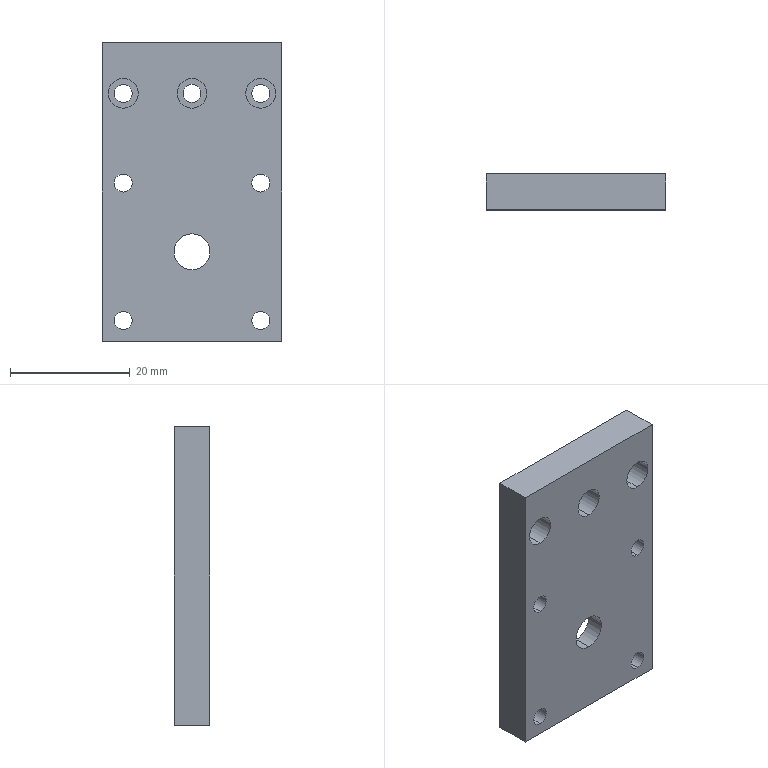Part | SolidWorks | features ICE 3, Cut 2, FlatPattern 1, SMBaseFlange 1, SheetMetal 1 | 1 solid | 34 faces | box 30 x 6 x 50 mm | volume 7901 mm3 | cylinder 24 | plane 10 | commonest cylinder face diameters 3 x14 5 x6 6 x2 15.5 x2
STEP:
#1=CARTESIAN_POINT('',(0.,-6.,14.));
#2=VERTEX_POINT('',#1);
#3=CARTESIAN_POINT('',(0.,-6.,19.));
#4=VERTEX_POINT('',#3);
#5=CARTESIAN_POINT('',(0.,-6.,16.5));
#6=DIRECTION('',(0.,1.,0.));
#7=DIRECTION('',(0.,0.,1.));
#8=AXIS2_PLACEMENT_3D('',#5,#6,#7);
#9=CIRCLE('',#8,2.5);
#10=EDGE_CURVE('',#2,#4,#9,.T.);
#11=ORIENTED_EDGE('',*,*,#10,.F.);
#12=CARTESIAN_POINT('',(0.,-2.,14.));
#13=VERTEX_POINT('',#12);
#14=CARTESIAN_POINT('',(0.,-6.,14.));
#15=DIRECTION('',(0.,1.,0.));
#16=VECTOR('',#15,1000.);
#17=LINE('',#14,#16);
#18=EDGE_CURVE('',#2,#13,#17,.T.);
#19=ORIENTED_EDGE('',*,*,#18,.T.);
#20=CARTESIAN_POINT('',(0.,-2.,19.));
#21=VERTEX_POINT('',#20);
#22=CARTESIAN_POINT('',(0.,-2.,16.5));
#23=DIRECTION('',(0.,1.,0.));
#24=DIRECTION('',(0.,0.,1.));
#25=AXIS2_PLACEMENT_3D('',#22,#23,#24);
#26=CIRCLE('',#25,2.5);
#27=EDGE_CURVE('',#13,#21,#26,.T.);
#28=ORIENTED_EDGE('',*,*,#27,.T.);
#29=CARTESIAN_POINT('',(0.,-6.,19.));
#30=DIRECTION('',(0.,1.,0.));
#31=VECTOR('',#30,1000.);
#32=LINE('',#29,#31);
#33=EDGE_CURVE('',#4,#21,#32,.T.);
#34=ORIENTED_EDGE('',*,*,#33,.F.);
#35=EDGE_LOOP('',(#11,#19,#28,#34));
#36=FACE_OUTER_BOUND('',#35,.T.);
#37=CARTESIAN_POINT('',(0.,-6.,16.5));
#38=DIRECTION('',(0.,1.,0.));
#39=DIRECTION('',(0.,0.,1.));
#40=AXIS2_PLACEMENT_3D('',#37,#38,#39);
#41=CYLINDRICAL_SURFACE('',#40,2.5);
#42=ADVANCED_FACE('',(#36),#41,.F.);
#43=CARTESIAN_POINT('',(11.5,-6.,14.));
#44=VERTEX_POINT('',#43);
#45=CARTESIAN_POINT('',(11.5,-6.,19.));
#46=VERTEX_POINT('',#45);
#47=CARTESIAN_POINT('',(11.5,-6.,16.5));
#48=DIRECTION('',(0.,1.,0.));
#49=DIRECTION('',(0.,0.,1.));
#50=AXIS2_PLACEMENT_3D('',#47,#48,#49);
#51=CIRCLE('',#50,2.5);
#52=EDGE_CURVE('',#44,#46,#51,.T.);
#53=ORIENTED_EDGE('',*,*,#52,.F.);
#54=CARTESIAN_POINT('',(11.5,-2.,14.));
#55=VERTEX_POINT('',#54);
#56=CARTESIAN_POINT('',(11.5,-6.,14.));
#57=DIRECTION('',(0.,1.,0.));
#58=VECTOR('',#57,1000.);
#59=LINE('',#56,#58);
#60=EDGE_CURVE('',#44,#55,#59,.T.);
#61=ORIENTED_EDGE('',*,*,#60,.T.);
#62=CARTESIAN_POINT('',(11.5,-2.,19.));
#63=VERTEX_POINT('',#62);
#64=CARTESIAN_POINT('',(11.5,-2.,16.5));
#65=DIRECTION('',(0.,1.,0.));
#66=DIRECTION('',(0.,0.,1.));
#67=AXIS2_PLACEMENT_3D('',#64,#65,#66);
#68=CIRCLE('',#67,2.5);
#69=EDGE_CURVE('',#55,#63,#68,.T.);
#70=ORIENTED_EDGE('',*,*,#69,.T.);
#71=CARTESIAN_POINT('',(11.5,-6.,19.));
#72=DIRECTION('',(0.,1.,0.));
#73=VECTOR('',#72,1000.);
#74=LINE('',#71,#73);
#75=EDGE_CURVE('',#46,#63,#74,.T.);
#76=ORIENTED_EDGE('',*,*,#75,.F.);
#77=EDGE_LOOP('',(#53,#61,#70,#76));
#78=FACE_OUTER_BOUND('',#77,.T.);
#79=CARTESIAN_POINT('',(11.5,-6.,16.5));
#80=DIRECTION('',(0.,1.,0.));
#81=DIRECTION('',(0.,0.,1.));
#82=AXIS2_PLACEMENT_3D('',#79,#80,#81);
#83=CYLINDRICAL_SURFACE('',#82,2.5);
#84=ADVANCED_FACE('',(#78),#83,.F.);
#85=CARTESIAN_POINT('',(-11.5,-6.,14.));
#86=VERTEX_POINT('',#85);
#87=CARTESIAN_POINT('',(-11.5,-6.,19.));
#88=VERTEX_POINT('',#87);
#89=CARTESIAN_POINT('',(-11.5,-6.,16.5));
#90=DIRECTION('',(0.,1.,0.));
#91=DIRECTION('',(0.,0.,1.));
#92=AXIS2_PLACEMENT_3D('',#89,#90,#91);
#93=CIRCLE('',#92,2.5);
#94=EDGE_CURVE('',#86,#88,#93,.T.);
#95=ORIENTED_EDGE('',*,*,#94,.F.);
#96=CARTESIAN_POINT('',(-11.5,-2.,14.));
#97=VERTEX_POINT('',#96);
#98=CARTESIAN_POINT('',(-11.5,-6.,14.));
#99=DIRECTION('',(0.,1.,0.));
#100=VECTOR('',#99,1000.);
#101=LINE('',#98,#100);
#102=EDGE_CURVE('',#86,#97,#101,.T.);
#103=ORIENTED_EDGE('',*,*,#102,.T.);
#104=CARTESIAN_POINT('',(-11.5,-2.,19.));
#105=VERTEX_POINT('',#104);
#106=CARTESIAN_POINT('',(-11.5,-2.,16.5));
#107=DIRECTION('',(0.,1.,0.));
#108=DIRECTION('',(0.,0.,1.));
#109=AXIS2_PLACEMENT_3D('',#106,#107,#108);
#110=CIRCLE('',#109,2.5);
#111=EDGE_CURVE('',#97,#105,#110,.T.);
#112=ORIENTED_EDGE('',*,*,#111,.T.);
#113=CARTESIAN_POINT('',(-11.5,-6.,19.));
#114=DIRECTION('',(0.,1.,0.));
#115=VECTOR('',#114,1000.);
#116=LINE('',#113,#115);
#117=EDGE_CURVE('',#88,#105,#116,.T.);
#118=ORIENTED_EDGE('',*,*,#117,.F.);
#119=EDGE_LOOP('',(#95,#103,#112,#118));
#120=FACE_OUTER_BOUND('',#119,.T.);
#121=CARTESIAN_POINT('',(-11.5,-6.,16.5));
#122=DIRECTION('',(0.,1.,0.));
#123=DIRECTION('',(0.,0.,1.));
#124=AXIS2_PLACEMENT_3D('',#121,#122,#123);
#125=CYLINDRICAL_SURFACE('',#124,2.5);
#126=ADVANCED_FACE('',(#120),#125,.F.);
#127=CARTESIAN_POINT('',(-11.5,-2.,18.));
#128=VERTEX_POINT('',#127);
#129=CARTESIAN_POINT('',(-11.5,-2.,15.));
#130=VERTEX_POINT('',#129);
#131=CARTESIAN_POINT('',(-11.5,-2.,16.5));
#132=DIRECTION('',(0.,-1.,0.));
#133=DIRECTION('',(0.,0.,1.));
#134=AXIS2_PLACEMENT_3D('',#131,#132,#133);
#135=CIRCLE('',#134,1.5);
#136=EDGE_CURVE('',#128,#130,#135,.T.);
#137=ORIENTED_EDGE('',*,*,#136,.T.);
#138=CARTESIAN_POINT('',(-11.5,0.,15.));
#139=VERTEX_POINT('',#138);
#140=CARTESIAN_POINT('',(-11.5,-6.,15.));
#141=DIRECTION('',(0.,1.,0.));
#142=VECTOR('',#141,1000.);
#143=LINE('',#140,#142);
#144=EDGE_CURVE('',#130,#139,#143,.T.);
#145=ORIENTED_EDGE('',*,*,#144,.T.);
#146=CARTESIAN_POINT('',(-11.5,0.,18.));
#147=VERTEX_POINT('',#146);
#148=CARTESIAN_POINT('',(-11.5,0.,16.5));
#149=DIRECTION('',(0.,1.,0.));
#150=DIRECTION('',(0.,0.,1.));
#151=AXIS2_PLACEMENT_3D('',#148,#149,#150);
#152=CIRCLE('',#151,1.5);
#153=EDGE_CURVE('',#139,#147,#152,.T.);
#154=ORIENTED_EDGE('',*,*,#153,.T.);
#155=CARTESIAN_POINT('',(-11.5,-6.,18.));
#156=DIRECTION('',(0.,1.,0.));
#157=VECTOR('',#156,1000.);
#158=LINE('',#155,#157);
#159=EDGE_CURVE('',#128,#147,#158,.T.);
#160=ORIENTED_EDGE('',*,*,#159,.F.);
#161=EDGE_LOOP('',(#137,#145,#154,#160));
#162=FACE_OUTER_BOUND('',#161,.T.);
#163=CARTESIAN_POINT('',(-11.5,-6.,16.5));
#164=DIRECTION('',(0.,1.,0.));
#165=DIRECTION('',(0.,0.,1.));
#166=AXIS2_PLACEMENT_3D('',#163,#164,#165);
#167=CYLINDRICAL_SURFACE('',#166,1.5);
#168=ADVANCED_FACE('',(#162),#167,.F.);
#169=CARTESIAN_POINT('',(11.5,-2.,18.));
#170=VERTEX_POINT('',#169);
#171=CARTESIAN_POINT('',(11.5,-2.,15.));
#172=VERTEX_POINT('',#171);
#173=CARTESIAN_POINT('',(11.5,-2.,16.5));
#174=DIRECTION('',(0.,-1.,0.));
#175=DIRECTION('',(0.,0.,1.));
#176=AXIS2_PLACEMENT_3D('',#173,#174,#175);
#177=CIRCLE('',#176,1.5);
#178=EDGE_CURVE('',#170,#172,#177,.T.);
#179=ORIENTED_EDGE('',*,*,#178,.T.);
#180=CARTESIAN_POINT('',(11.5,0.,15.));
#181=VERTEX_POINT('',#180);
#182=CARTESIAN_POINT('',(11.5,-6.,15.));
#183=DIRECTION('',(0.,1.,0.));
#184=VECTOR('',#183,1000.);
#185=LINE('',#182,#184);
#186=EDGE_CURVE('',#172,#181,#185,.T.);
#187=ORIENTED_EDGE('',*,*,#186,.T.);
#188=CARTESIAN_POINT('',(11.5,0.,18.));
#189=VERTEX_POINT('',#188);
#190=CARTESIAN_POINT('',(11.5,0.,16.5));
#191=DIRECTION('',(0.,1.,0.));
#192=DIRECTION('',(0.,0.,1.));
#193=AXIS2_PLACEMENT_3D('',#190,#191,#192);
#194=CIRCLE('',#193,1.5);
#195=EDGE_CURVE('',#181,#189,#194,.T.);
#196=ORIENTED_EDGE('',*,*,#195,.T.);
#197=CARTESIAN_POINT('',(11.5,-6.,18.));
#198=DIRECTION('',(0.,1.,0.));
#199=VECTOR('',#198,1000.);
#200=LINE('',#197,#199);
#201=EDGE_CURVE('',#170,#189,#200,.T.);
#202=ORIENTED_EDGE('',*,*,#201,.F.);
#203=EDGE_LOOP('',(#179,#187,#196,#202));
#204=FACE_OUTER_BOUND('',#203,.T.);
#205=CARTESIAN_POINT('',(11.5,-6.,16.5));
#206=DIRECTION('',(0.,1.,0.));
#207=DIRECTION('',(0.,0.,1.));
#208=AXIS2_PLACEMENT_3D('',#205,#206,#207);
#209=CYLINDRICAL_SURFACE('',#208,1.5);
#210=ADVANCED_FACE('',(#204),#209,.F.);
#211=CARTESIAN_POINT('',(0.,-2.,18.));
#212=VERTEX_POINT('',#211);
#213=CARTESIAN_POINT('',(0.,-2.,15.));
#214=VERTEX_POINT('',#213);
#215=CARTESIAN_POINT('',(0.,-2.,16.5));
#216=DIRECTION('',(0.,-1.,0.));
#217=DIRECTION('',(0.,0.,1.));
#218=AXIS2_PLACEMENT_3D('',#215,#216,#217);
#219=CIRCLE('',#218,1.5);
#220=EDGE_CURVE('',#212,#214,#219,.T.);
#221=ORIENTED_EDGE('',*,*,#220,.T.);
#222=CARTESIAN_POINT('',(0.,0.,15.));
#223=VERTEX_POINT('',#222);
#224=CARTESIAN_POINT('',(0.,-6.,15.));
#225=DIRECTION('',(0.,1.,0.));
#226=VECTOR('',#225,1000.);
#227=LINE('',#224,#226);
#228=EDGE_CURVE('',#214,#223,#227,.T.);
#229=ORIENTED_EDGE('',*,*,#228,.T.);
#230=CARTESIAN_POINT('',(0.,0.,18.));
#231=VERTEX_POINT('',#230);
#232=CARTESIAN_POINT('',(0.,0.,16.5));
#233=DIRECTION('',(0.,1.,0.));
#234=DIRECTION('',(0.,0.,1.));
#235=AXIS2_PLACEMENT_3D('',#232,#233,#234);
#236=CIRCLE('',#235,1.5);
#237=EDGE_CURVE('',#223,#231,#236,.T.);
#238=ORIENTED_EDGE('',*,*,#237,.T.);
#239=CARTESIAN_POINT('',(0.,-6.,18.));
#240=DIRECTION('',(0.,1.,0.));
#241=VECTOR('',#240,1000.);
#242=LINE('',#239,#241);
#243=EDGE_CURVE('',#212,#231,#242,.T.);
#244=ORIENTED_EDGE('',*,*,#243,.F.);
#245=EDGE_LOOP('',(#221,#229,#238,#244));
#246=FACE_OUTER_BOUND('',#245,.T.);
#247=CARTESIAN_POINT('',(0.,-6.,16.5));
#248=DIRECTION('',(0.,1.,0.));
#249=DIRECTION('',(0.,0.,1.));
#250=AXIS2_PLACEMENT_3D('',#247,#248,#249);
#251=CYLINDRICAL_SURFACE('',#250,1.5);
#252=ADVANCED_FACE('',(#246),#251,.F.);
#253=CARTESIAN_POINT('',(0.,-3.,-17.75));
#254=VERTEX_POINT('',#253);
#255=CARTESIAN_POINT('',(0.,-3.,-2.25));
#256=VERTEX_POINT('',#255);
#257=CARTESIAN_POINT('',(0.,-3.,-10.));
#258=DIRECTION('',(0.,1.,0.));
#259=DIRECTION('',(0.,0.,1.));
#260=AXIS2_PLACEMENT_3D('',#257,#258,#259);
#261=CIRCLE('',#260,7.75);
#262=EDGE_CURVE('',#254,#256,#261,.T.);
#263=ORIENTED_EDGE('',*,*,#262,.F.);
#264=CARTESIAN_POINT('',(0.,0.,-17.75));
#265=VERTEX_POINT('',#264);
#266=CARTESIAN_POINT('',(0.,-3.,-17.75));
#267=DIRECTION('',(0.,1.,0.));
#268=VECTOR('',#267,1000.);
#269=LINE('',#266,#268);
#270=EDGE_CURVE('',#254,#265,#269,.T.);
#271=ORIENTED_EDGE('',*,*,#270,.T.);
#272=CARTESIAN_POINT('',(0.,0.,-2.25));
#273=VERTEX_POINT('',#272);
#274=CARTESIAN_POINT('',(0.,0.,-10.));
#275=DIRECTION('',(0.,1.,0.));
#276=DIRECTION('',(0.,0.,1.));
#277=AXIS2_PLACEMENT_3D('',#274,#275,#276);
#278=CIRCLE('',#277,7.75);
#279=EDGE_CURVE('',#265,#273,#278,.T.);
#280=ORIENTED_EDGE('',*,*,#279,.T.);
#281=CARTESIAN_POINT('',(0.,-3.,-2.25));
#282=DIRECTION('',(0.,1.,0.));
#283=VECTOR('',#282,1000.);
#284=LINE('',#281,#283);
#285=EDGE_CURVE('',#256,#273,#284,.T.);
#286=ORIENTED_EDGE('',*,*,#285,.F.);
#287=EDGE_LOOP('',(#263,#271,#280,#286));
#288=FACE_OUTER_BOUND('',#287,.T.);
#289=CARTESIAN_POINT('',(0.,-3.,-10.));
#290=DIRECTION('',(0.,1.,0.));
#291=DIRECTION('',(0.,0.,1.));
#292=AXIS2_PLACEMENT_3D('',#289,#290,#291);
#293=CYLINDRICAL_SURFACE('',#292,7.75);
#294=ADVANCED_FACE('',(#288),#293,.F.);
#295=CARTESIAN_POINT('',(11.5,0.,3.));
#296=VERTEX_POINT('',#295);
#297=CARTESIAN_POINT('',(11.5,0.,0.));
#298=VERTEX_POINT('',#297);
#299=CARTESIAN_POINT('',(11.5,0.,1.5));
#300=DIRECTION('',(0.,-1.,0.));
#301=DIRECTION('',(0.,0.,-1.));
#302=AXIS2_PLACEMENT_3D('',#299,#300,#301);
#303=CIRCLE('',#302,1.5);
#304=EDGE_CURVE('',#296,#298,#303,.T.);
#305=ORIENTED_EDGE('',*,*,#304,.F.);
#306=CARTESIAN_POINT('',(11.5,-6.,3.));
#307=VERTEX_POINT('',#306);
#308=CARTESIAN_POINT('',(11.5,0.,3.));
#309=DIRECTION('',(0.,-1.,0.));
#310=VECTOR('',#309,1000.);
#311=LINE('',#308,#310);
#312=EDGE_CURVE('',#296,#307,#311,.T.);
#313=ORIENTED_EDGE('',*,*,#312,.T.);
#314=CARTESIAN_POINT('',(11.5,-6.,0.));
#315=VERTEX_POINT('',#314);
#316=CARTESIAN_POINT('',(11.5,-6.,1.5));
#317=DIRECTION('',(0.,-1.,0.));
#318=DIRECTION('',(0.,0.,-1.));
#319=AXIS2_PLACEMENT_3D('',#316,#317,#318);
#320=CIRCLE('',#319,1.5);
#321=EDGE_CURVE('',#307,#315,#320,.T.);
#322=ORIENTED_EDGE('',*,*,#321,.T.);
#323=CARTESIAN_POINT('',(11.5,0.,0.));
#324=DIRECTION('',(0.,-1.,0.));
#325=VECTOR('',#324,1000.);
#326=LINE('',#323,#325);
#327=EDGE_CURVE('',#298,#315,#326,.T.);
#328=ORIENTED_EDGE('',*,*,#327,.F.);
#329=EDGE_LOOP('',(#305,#313,#322,#328));
#330=FACE_OUTER_BOUND('',#329,.T.);
#331=CARTESIAN_POINT('',(11.5,0.,1.5));
#332=DIRECTION('',(0.,-1.,0.));
#333=DIRECTION('',(0.,0.,-1.));
#334=AXIS2_PLACEMENT_3D('',#331,#332,#333);
#335=CYLINDRICAL_SURFACE('',#334,1.5);
#336=ADVANCED_FACE('',(#330),#335,.F.);
#337=CARTESIAN_POINT('',(-11.5,0.,3.));
#338=VERTEX_POINT('',#337);
#339=CARTESIAN_POINT('',(-11.5,0.,0.));
#340=VERTEX_POINT('',#339);
#341=CARTESIAN_POINT('',(-11.5,0.,1.5));
#342=DIRECTION('',(0.,-1.,0.));
#343=DIRECTION('',(0.,0.,-1.));
#344=AXIS2_PLACEMENT_3D('',#341,#342,#343);
#345=CIRCLE('',#344,1.5);
#346=EDGE_CURVE('',#338,#340,#345,.T.);
#347=ORIENTED_EDGE('',*,*,#346,.F.);
#348=CARTESIAN_POINT('',(-11.5,-6.,3.));
#349=VERTEX_POINT('',#348);
#350=CARTESIAN_POINT('',(-11.5,0.,3.));
#351=DIRECTION('',(0.,-1.,0.));
#352=VECTOR('',#351,1000.);
#353=LINE('',#350,#352);
#354=EDGE_CURVE('',#338,#349,#353,.T.);
#355=ORIENTED_EDGE('',*,*,#354,.T.);
#356=CARTESIAN_POINT('',(-11.5,-6.,0.));
#357=VERTEX_POINT('',#356);
#358=CARTESIAN_POINT('',(-11.5,-6.,1.5));
#359=DIRECTION('',(0.,-1.,0.));
#360=DIRECTION('',(0.,0.,-1.));
#361=AXIS2_PLACEMENT_3D('',#358,#359,#360);
#362=CIRCLE('',#361,1.5);
#363=EDGE_CURVE('',#349,#357,#362,.T.);
#364=ORIENTED_EDGE('',*,*,#363,.T.);
#365=CARTESIAN_POINT('',(-11.5,0.,0.));
#366=DIRECTION('',(0.,-1.,0.));
#367=VECTOR('',#366,1000.);
#368=LINE('',#365,#367);
#369=EDGE_CURVE('',#340,#357,#368,.T.);
#370=ORIENTED_EDGE('',*,*,#369,.F.);
#371=EDGE_LOOP('',(#347,#355,#364,#370));
#372=FACE_OUTER_BOUND('',#371,.T.);
#373=CARTESIAN_POINT('',(-11.5,0.,1.5));
#374=DIRECTION('',(0.,-1.,0.));
#375=DIRECTION('',(0.,0.,-1.));
#376=AXIS2_PLACEMENT_3D('',#373,#374,#375);
#377=CYLINDRICAL_SURFACE('',#376,1.5);
#378=ADVANCED_FACE('',(#372),#377,.F.);
#379=CARTESIAN_POINT('',(-11.5,0.,-20.));
#380=VERTEX_POINT('',#379);
#381=CARTESIAN_POINT('',(-11.5,0.,-23.));
#382=VERTEX_POINT('',#381);
#383=CARTESIAN_POINT('',(-11.5,0.,-21.5));
#384=DIRECTION('',(0.,-1.,0.));
#385=DIRECTION('',(0.,0.,-1.));
#386=AXIS2_PLACEMENT_3D('',#383,#384,#385);
#387=CIRCLE('',#386,1.5);
#388=EDGE_CURVE('',#380,#382,#387,.T.);
#389=ORIENTED_EDGE('',*,*,#388,.F.);
#390=CARTESIAN_POINT('',(-11.5,-6.,-20.));
#391=VERTEX_POINT('',#390);
#392=CARTESIAN_POINT('',(-11.5,0.,-20.));
#393=DIRECTION('',(0.,-1.,0.));
#394=VECTOR('',#393,1000.);
#395=LINE('',#392,#394);
#396=EDGE_CURVE('',#380,#391,#395,.T.);
#397=ORIENTED_EDGE('',*,*,#396,.T.);
#398=CARTESIAN_POINT('',(-11.5,-6.,-23.));
#399=VERTEX_POINT('',#398);
#400=CARTESIAN_POINT('',(-11.5,-6.,-21.5));
#401=DIRECTION('',(0.,-1.,0.));
#402=DIRECTION('',(0.,0.,-1.));
#403=AXIS2_PLACEMENT_3D('',#400,#401,#402);
#404=CIRCLE('',#403,1.5);
#405=EDGE_CURVE('',#391,#399,#404,.T.);
#406=ORIENTED_EDGE('',*,*,#405,.T.);
#407=CARTESIAN_POINT('',(-11.5,0.,-23.));
#408=DIRECTION('',(0.,-1.,0.));
#409=VECTOR('',#408,1000.);
#410=LINE('',#407,#409);
#411=EDGE_CURVE('',#382,#399,#410,.T.);
#412=ORIENTED_EDGE('',*,*,#411,.F.);
#413=EDGE_LOOP('',(#389,#397,#406,#412));
#414=FACE_OUTER_BOUND('',#413,.T.);
#415=CARTESIAN_POINT('',(-11.5,0.,-21.5));
#416=DIRECTION('',(0.,-1.,0.));
#417=DIRECTION('',(0.,0.,-1.));
#418=AXIS2_PLACEMENT_3D('',#415,#416,#417);
#419=CYLINDRICAL_SURFACE('',#418,1.5);
#420=ADVANCED_FACE('',(#414),#419,.F.);
#421=CARTESIAN_POINT('',(11.5,0.,-20.));
#422=VERTEX_POINT('',#421);
#423=CARTESIAN_POINT('',(11.5,0.,-23.));
#424=VERTEX_POINT('',#423);
#425=CARTESIAN_POINT('',(11.5,0.,-21.5));
#426=DIRECTION('',(0.,-1.,0.));
#427=DIRECTION('',(0.,0.,-1.));
#428=AXIS2_PLACEMENT_3D('',#425,#426,#427);
#429=CIRCLE('',#428,1.5);
#430=EDGE_CURVE('',#422,#424,#429,.T.);
#431=ORIENTED_EDGE('',*,*,#430,.F.);
#432=CARTESIAN_POINT('',(11.5,-6.,-20.));
#433=VERTEX_POINT('',#432);
#434=CARTESIAN_POINT('',(11.5,0.,-20.));
#435=DIRECTION('',(0.,-1.,0.));
#436=VECTOR('',#435,1000.);
#437=LINE('',#434,#436);
#438=EDGE_CURVE('',#422,#433,#437,.T.);
#439=ORIENTED_EDGE('',*,*,#438,.T.);
#440=CARTESIAN_POINT('',(11.5,-6.,-23.));
#441=VERTEX_POINT('',#440);
#442=CARTESIAN_POINT('',(11.5,-6.,-21.5));
#443=DIRECTION('',(0.,-1.,0.));
#444=DIRECTION('',(0.,0.,-1.));
#445=AXIS2_PLACEMENT_3D('',#442,#443,#444);
#446=CIRCLE('',#445,1.5);
#447=EDGE_CURVE('',#433,#441,#446,.T.);
#448=ORIENTED_EDGE('',*,*,#447,.T.);
#449=CARTESIAN_POINT('',(11.5,0.,-23.));
#450=DIRECTION('',(0.,-1.,0.));
#451=VECTOR('',#450,1000.);
#452=LINE('',#449,#451);
#453=EDGE_CURVE('',#424,#441,#452,.T.);
#454=ORIENTED_EDGE('',*,*,#453,.F.);
#455=EDGE_LOOP('',(#431,#439,#448,#454));
#456=FACE_OUTER_BOUND('',#455,.T.);
#457=CARTESIAN_POINT('',(11.5,0.,-21.5));
#458=DIRECTION('',(0.,-1.,0.));
#459=DIRECTION('',(0.,0.,-1.));
#460=AXIS2_PLACEMENT_3D('',#457,#458,#459);
#461=CYLINDRICAL_SURFACE('',#460,1.5);
#462=ADVANCED_FACE('',(#456),#461,.F.);
#463=CARTESIAN_POINT('',(0.,-3.,-7.));
#464=VERTEX_POINT('',#463);
#465=CARTESIAN_POINT('',(0.,-3.,-13.));
#466=VERTEX_POINT('',#465);
#467=CARTESIAN_POINT('',(0.,-3.,-10.));
#468=DIRECTION('',(0.,-1.,0.));
#469=DIRECTION('',(0.,0.,1.));
#470=AXIS2_PLACEMENT_3D('',#467,#468,#469);
#471=CIRCLE('',#470,3.);
#472=EDGE_CURVE('',#464,#466,#471,.T.);
#473=ORIENTED_EDGE('',*,*,#472,.F.);
#474=CARTESIAN_POINT('',(0.,-6.,-7.));
#475=VERTEX_POINT('',#474);
#476=CARTESIAN_POINT('',(0.,0.,-7.));
#477=DIRECTION('',(0.,-1.,0.));
#478=VECTOR('',#477,1000.);
#479=LINE('',#476,#478);
#480=EDGE_CURVE('',#464,#475,#479,.T.);
#481=ORIENTED_EDGE('',*,*,#480,.T.);
#482=CARTESIAN_POINT('',(0.,-6.,-13.));
#483=VERTEX_POINT('',#482);
#484=CARTESIAN_POINT('',(0.,-6.,-10.));
#485=DIRECTION('',(0.,-1.,0.));
#486=DIRECTION('',(0.,0.,-1.));
#487=AXIS2_PLACEMENT_3D('',#484,#485,#486);
#488=CIRCLE('',#487,3.);
#489=EDGE_CURVE('',#475,#483,#488,.T.);
#490=ORIENTED_EDGE('',*,*,#489,.T.);
#491=CARTESIAN_POINT('',(0.,0.,-13.));
#492=DIRECTION('',(0.,-1.,0.));
#493=VECTOR('',#492,1000.);
#494=LINE('',#491,#493);
#495=EDGE_CURVE('',#466,#483,#494,.T.);
#496=ORIENTED_EDGE('',*,*,#495,.F.);
#497=EDGE_LOOP('',(#473,#481,#490,#496));
#498=FACE_OUTER_BOUND('',#497,.T.);
#499=CARTESIAN_POINT('',(0.,0.,-10.));
#500=DIRECTION('',(0.,-1.,0.));
#501=DIRECTION('',(0.,0.,-1.));
#502=AXIS2_PLACEMENT_3D('',#499,#500,#501);
#503=CYLINDRICAL_SURFACE('',#502,3.);
#504=ADVANCED_FACE('',(#498),#503,.F.);
#505=ORIENTED_EDGE('',*,*,#480,.F.);
#506=CARTESIAN_POINT('',(0.,-3.,-10.));
#507=DIRECTION('',(0.,-1.,0.));
#508=DIRECTION('',(0.,0.,1.));
#509=AXIS2_PLACEMENT_3D('',#506,#507,#508);
#510=CIRCLE('',#509,3.);
#511=EDGE_CURVE('',#466,#464,#510,.T.);
#512=ORIENTED_EDGE('',*,*,#511,.F.);
#513=ORIENTED_EDGE('',*,*,#495,.T.);
#514=CARTESIAN_POINT('',(0.,-6.,-10.));
#515=DIRECTION('',(0.,-1.,0.));
#516=DIRECTION('',(0.,0.,-1.));
#517=AXIS2_PLACEMENT_3D('',#514,#515,#516);
#518=CIRCLE('',#517,3.);
#519=EDGE_CURVE('',#483,#475,#518,.T.);
#520=ORIENTED_EDGE('',*,*,#519,.T.);
#521=EDGE_LOOP('',(#505,#512,#513,#520));
#522=FACE_OUTER_BOUND('',#521,.T.);
#523=CARTESIAN_POINT('',(0.,0.,-10.));
#524=DIRECTION('',(0.,-1.,0.));
#525=DIRECTION('',(0.,0.,-1.));
#526=AXIS2_PLACEMENT_3D('',#523,#524,#525);
#527=CYLINDRICAL_SURFACE('',#526,3.);
#528=ADVANCED_FACE('',(#522),#527,.F.);
#529=CARTESIAN_POINT('',(15.,0.,25.));
#530=VERTEX_POINT('',#529);
#531=CARTESIAN_POINT('',(15.,0.,-25.));
#532=VERTEX_POINT('',#531);
#533=CARTESIAN_POINT('',(15.,0.,-25.));
#534=DIRECTION('',(0.,0.,-1.));
#535=VECTOR('',#534,1000.);
#536=LINE('',#533,#535);
#537=EDGE_CURVE('',#530,#532,#536,.T.);
#538=ORIENTED_EDGE('',*,*,#537,.F.);
#539=CARTESIAN_POINT('',(15.,-6.,25.));
#540=VERTEX_POINT('',#539);
#541=CARTESIAN_POINT('',(15.,-6.,25.));
#542=DIRECTION('',(0.,1.,0.));
#543=VECTOR('',#542,1000.);
#544=LINE('',#541,#543);
#545=EDGE_CURVE('',#540,#530,#544,.T.);
#546=ORIENTED_EDGE('',*,*,#545,.F.);
#547=CARTESIAN_POINT('',(15.,-6.,-25.));
#548=VERTEX_POINT('',#547);
#549=CARTESIAN_POINT('',(15.,-6.,-25.));
#550=DIRECTION('',(0.,0.,-1.));
#551=VECTOR('',#550,1000.);
#552=LINE('',#549,#551);
#553=EDGE_CURVE('',#540,#548,#552,.T.);
#554=ORIENTED_EDGE('',*,*,#553,.T.);
#555=CARTESIAN_POINT('',(15.,-6.,-25.));
#556=DIRECTION('',(0.,1.,0.));
#557=VECTOR('',#556,1000.);
#558=LINE('',#555,#557);
#559=EDGE_CURVE('',#548,#532,#558,.T.);
#560=ORIENTED_EDGE('',*,*,#559,.T.);
#561=EDGE_LOOP('',(#538,#546,#554,#560));
#562=FACE_OUTER_BOUND('',#561,.T.);
#563=CARTESIAN_POINT('',(15.,-6.,-25.));
#564=DIRECTION('',(1.,0.,0.));
#565=DIRECTION('',(0.,0.,-1.));
#566=AXIS2_PLACEMENT_3D('',#563,#564,#565);
#567=PLANE('',#566);
#568=ADVANCED_FACE('',(#562),#567,.T.);
#569=CARTESIAN_POINT('',(-15.,0.,25.));
#570=VERTEX_POINT('',#569);
#571=CARTESIAN_POINT('',(-15.,0.,25.));
#572=DIRECTION('',(1.,0.,0.));
#573=VECTOR('',#572,1000.);
#574=LINE('',#571,#573);
#575=EDGE_CURVE('',#570,#530,#574,.T.);
#576=ORIENTED_EDGE('',*,*,#575,.F.);
#577=CARTESIAN_POINT('',(-15.,-6.,25.));
#578=VERTEX_POINT('',#577);
#579=CARTESIAN_POINT('',(-15.,-6.,25.));
#580=DIRECTION('',(0.,1.,0.));
#581=VECTOR('',#580,1000.);
#582=LINE('',#579,#581);
#583=EDGE_CURVE('',#578,#570,#582,.T.);
#584=ORIENTED_EDGE('',*,*,#583,.F.);
#585=CARTESIAN_POINT('',(-15.,-6.,25.));
#586=DIRECTION('',(1.,0.,0.));
#587=VECTOR('',#586,1000.);
#588=LINE('',#585,#587);
#589=EDGE_CURVE('',#578,#540,#588,.T.);
#590=ORIENTED_EDGE('',*,*,#589,.T.);
#591=ORIENTED_EDGE('',*,*,#545,.T.);
#592=EDGE_LOOP('',(#576,#584,#590,#591));
#593=FACE_OUTER_BOUND('',#592,.T.);
#594=CARTESIAN_POINT('',(-15.,-6.,25.));
#595=DIRECTION('',(0.,0.,1.));
#596=DIRECTION('',(1.,0.,0.));
#597=AXIS2_PLACEMENT_3D('',#594,#595,#596);
#598=PLANE('',#597);
#599=ADVANCED_FACE('',(#593),#598,.T.);
#600=CARTESIAN_POINT('',(-15.,0.,-25.));
#601=VERTEX_POINT('',#600);
#602=CARTESIAN_POINT('',(-15.,0.,-25.));
#603=DIRECTION('',(0.,0.,1.));
#604=VECTOR('',#603,1000.);
#605=LINE('',#602,#604);
#606=EDGE_CURVE('',#601,#570,#605,.T.);
#607=ORIENTED_EDGE('',*,*,#606,.F.);
#608=CARTESIAN_POINT('',(-15.,-6.,-25.));
#609=VERTEX_POINT('',#608);
#610=CARTESIAN_POINT('',(-15.,-6.,-25.));
#611=DIRECTION('',(0.,1.,0.));
#612=VECTOR('',#611,1000.);
#613=LINE('',#610,#612);
#614=EDGE_CURVE('',#609,#601,#613,.T.);
#615=ORIENTED_EDGE('',*,*,#614,.F.);
#616=CARTESIAN_POINT('',(-15.,-6.,-25.));
#617=DIRECTION('',(0.,0.,1.));
#618=VECTOR('',#617,1000.);
#619=LINE('',#616,#618);
#620=EDGE_CURVE('',#609,#578,#619,.T.);
#621=ORIENTED_EDGE('',*,*,#620,.T.);
#622=ORIENTED_EDGE('',*,*,#583,.T.);
#623=EDGE_LOOP('',(#607,#615,#621,#622));
#624=FACE_OUTER_BOUND('',#623,.T.);
#625=CARTESIAN_POINT('',(-15.,-6.,-25.));
#626=DIRECTION('',(-1.,0.,0.));
#627=DIRECTION('',(0.,0.,1.));
#628=AXIS2_PLACEMENT_3D('',#625,#626,#627);
#629=PLANE('',#628);
#630=ADVANCED_FACE('',(#624),#629,.T.);
#631=CARTESIAN_POINT('',(-15.,0.,-25.));
#632=DIRECTION('',(-1.,0.,0.));
#633=VECTOR('',#632,1000.);
#634=LINE('',#631,#633);
#635=EDGE_CURVE('',#532,#601,#634,.T.);
#636=ORIENTED_EDGE('',*,*,#635,.F.);
#637=ORIENTED_EDGE('',*,*,#559,.F.);
#638=CARTESIAN_POINT('',(-15.,-6.,-25.));
#639=DIRECTION('',(-1.,0.,0.));
#640=VECTOR('',#639,1000.);
#641=LINE('',#638,#640);
#642=EDGE_CURVE('',#548,#609,#641,.T.);
#643=ORIENTED_EDGE('',*,*,#642,.T.);
#644=ORIENTED_EDGE('',*,*,#614,.T.);
#645=EDGE_LOOP('',(#636,#637,#643,#644));
#646=FACE_OUTER_BOUND('',#645,.T.);
#647=CARTESIAN_POINT('',(-15.,-6.,-25.));
#648=DIRECTION('',(0.,0.,-1.));
#649=DIRECTION('',(-1.,0.,0.));
#650=AXIS2_PLACEMENT_3D('',#647,#648,#649);
#651=PLANE('',#650);
#652=ADVANCED_FACE('',(#646),#651,.T.);
#653=CARTESIAN_POINT('',(11.5,-6.,16.5));
#654=DIRECTION('',(0.,1.,0.));
#655=DIRECTION('',(0.,0.,1.));
#656=AXIS2_PLACEMENT_3D('',#653,#654,#655);
#657=CIRCLE('',#656,2.5);
#658=EDGE_CURVE('',#46,#44,#657,.T.);
#659=ORIENTED_EDGE('',*,*,#658,.T.);
#660=ORIENTED_EDGE('',*,*,#52,.T.);
#661=EDGE_LOOP('',(#659,#660));
#662=FACE_BOUND('',#661,.T.);
#663=CARTESIAN_POINT('',(-11.5,-6.,16.5));
#664=DIRECTION('',(0.,1.,0.));
#665=DIRECTION('',(0.,0.,1.));
#666=AXIS2_PLACEMENT_3D('',#663,#664,#665);
#667=CIRCLE('',#666,2.5);
#668=EDGE_CURVE('',#88,#86,#667,.T.);
#669=ORIENTED_EDGE('',*,*,#668,.T.);
#670=ORIENTED_EDGE('',*,*,#94,.T.);
#671=EDGE_LOOP('',(#669,#670));
#672=FACE_BOUND('',#671,.T.);
#673=CARTESIAN_POINT('',(0.,-6.,16.5));
#674=DIRECTION('',(0.,1.,0.));
#675=DIRECTION('',(0.,0.,1.));
#676=AXIS2_PLACEMENT_3D('',#673,#674,#675);
#677=CIRCLE('',#676,2.5);
#678=EDGE_CURVE('',#4,#2,#677,.T.);
#679=ORIENTED_EDGE('',*,*,#678,.T.);
#680=ORIENTED_EDGE('',*,*,#10,.T.);
#681=EDGE_LOOP('',(#679,#680));
#682=FACE_BOUND('',#681,.T.);
#683=ORIENTED_EDGE('',*,*,#519,.F.);
#684=ORIENTED_EDGE('',*,*,#489,.F.);
#685=EDGE_LOOP('',(#683,#684));
#686=FACE_BOUND('',#685,.T.);
#687=CARTESIAN_POINT('',(11.5,-6.,1.5));
#688=DIRECTION('',(0.,-1.,0.));
#689=DIRECTION('',(0.,0.,-1.));
#690=AXIS2_PLACEMENT_3D('',#687,#688,#689);
#691=CIRCLE('',#690,1.5);
#692=EDGE_CURVE('',#315,#307,#691,.T.);
#693=ORIENTED_EDGE('',*,*,#692,.F.);
#694=ORIENTED_EDGE('',*,*,#321,.F.);
#695=EDGE_LOOP('',(#693,#694));
#696=FACE_BOUND('',#695,.T.);
#697=CARTESIAN_POINT('',(-11.5,-6.,1.5));
#698=DIRECTION('',(0.,-1.,0.));
#699=DIRECTION('',(0.,0.,-1.));
#700=AXIS2_PLACEMENT_3D('',#697,#698,#699);
#701=CIRCLE('',#700,1.5);
#702=EDGE_CURVE('',#357,#349,#701,.T.);
#703=ORIENTED_EDGE('',*,*,#702,.F.);
#704=ORIENTED_EDGE('',*,*,#363,.F.);
#705=EDGE_LOOP('',(#703,#704));
#706=FACE_BOUND('',#705,.T.);
#707=CARTESIAN_POINT('',(-11.5,-6.,-21.5));
#708=DIRECTION('',(0.,-1.,0.));
#709=DIRECTION('',(0.,0.,-1.));
#710=AXIS2_PLACEMENT_3D('',#707,#708,#709);
#711=CIRCLE('',#710,1.5);
#712=EDGE_CURVE('',#399,#391,#711,.T.);
#713=ORIENTED_EDGE('',*,*,#712,.F.);
#714=ORIENTED_EDGE('',*,*,#405,.F.);
#715=EDGE_LOOP('',(#713,#714));
#716=FACE_BOUND('',#715,.T.);
#717=CARTESIAN_POINT('',(11.5,-6.,-21.5));
#718=DIRECTION('',(0.,-1.,0.));
#719=DIRECTION('',(0.,0.,-1.));
#720=AXIS2_PLACEMENT_3D('',#717,#718,#719);
#721=CIRCLE('',#720,1.5);
#722=EDGE_CURVE('',#441,#433,#721,.T.);
#723=ORIENTED_EDGE('',*,*,#722,.F.);
#724=ORIENTED_EDGE('',*,*,#447,.F.);
#725=EDGE_LOOP('',(#723,#724));
#726=FACE_BOUND('',#725,.T.);
#727=ORIENTED_EDGE('',*,*,#553,.F.);
#728=ORIENTED_EDGE('',*,*,#589,.F.);
#729=ORIENTED_EDGE('',*,*,#620,.F.);
#730=ORIENTED_EDGE('',*,*,#642,.F.);
#731=EDGE_LOOP('',(#727,#728,#729,#730));
#732=FACE_OUTER_BOUND('',#731,.T.);
#733=CARTESIAN_POINT('',(0.,-6.,0.));
#734=DIRECTION('',(0.,1.,0.));
#735=DIRECTION('',(0.,0.,1.));
#736=AXIS2_PLACEMENT_3D('',#733,#734,#735);
#737=PLANE('',#736);
#738=ADVANCED_FACE('',(#662,#672,#682,#686,#696,#706,#716,#726,#732),#737,.F.);
#739=CARTESIAN_POINT('',(-11.5,0.,16.5));
#740=DIRECTION('',(0.,1.,0.));
#741=DIRECTION('',(0.,0.,1.));
#742=AXIS2_PLACEMENT_3D('',#739,#740,#741);
#743=CIRCLE('',#742,1.5);
#744=EDGE_CURVE('',#147,#139,#743,.T.);
#745=ORIENTED_EDGE('',*,*,#744,.F.);
#746=ORIENTED_EDGE('',*,*,#153,.F.);
#747=EDGE_LOOP('',(#745,#746));
#748=FACE_BOUND('',#747,.T.);
#749=CARTESIAN_POINT('',(11.5,0.,16.5));
#750=DIRECTION('',(0.,1.,0.));
#751=DIRECTION('',(0.,0.,1.));
#752=AXIS2_PLACEMENT_3D('',#749,#750,#751);
#753=CIRCLE('',#752,1.5);
#754=EDGE_CURVE('',#189,#181,#753,.T.);
#755=ORIENTED_EDGE('',*,*,#754,.F.);
#756=ORIENTED_EDGE('',*,*,#195,.F.);
#757=EDGE_LOOP('',(#755,#756));
#758=FACE_BOUND('',#757,.T.);
#759=CARTESIAN_POINT('',(0.,0.,16.5));
#760=DIRECTION('',(0.,1.,0.));
#761=DIRECTION('',(0.,0.,1.));
#762=AXIS2_PLACEMENT_3D('',#759,#760,#761);
#763=CIRCLE('',#762,1.5);
#764=EDGE_CURVE('',#231,#223,#763,.T.);
#765=ORIENTED_EDGE('',*,*,#764,.F.);
#766=ORIENTED_EDGE('',*,*,#237,.F.);
#767=EDGE_LOOP('',(#765,#766));
#768=FACE_BOUND('',#767,.T.);
#769=CARTESIAN_POINT('',(0.,0.,-10.));
#770=DIRECTION('',(0.,1.,0.));
#771=DIRECTION('',(0.,0.,1.));
#772=AXIS2_PLACEMENT_3D('',#769,#770,#771);
#773=CIRCLE('',#772,7.75);
#774=EDGE_CURVE('',#273,#265,#773,.T.);
#775=ORIENTED_EDGE('',*,*,#774,.F.);
#776=ORIENTED_EDGE('',*,*,#279,.F.);
#777=EDGE_LOOP('',(#775,#776));
#778=FACE_BOUND('',#777,.T.);
#779=CARTESIAN_POINT('',(11.5,0.,1.5));
#780=DIRECTION('',(0.,-1.,0.));
#781=DIRECTION('',(0.,0.,-1.));
#782=AXIS2_PLACEMENT_3D('',#779,#780,#781);
#783=CIRCLE('',#782,1.5);
#784=EDGE_CURVE('',#298,#296,#783,.T.);
#785=ORIENTED_EDGE('',*,*,#784,.T.);
#786=ORIENTED_EDGE('',*,*,#304,.T.);
#787=EDGE_LOOP('',(#785,#786));
#788=FACE_BOUND('',#787,.T.);
#789=CARTESIAN_POINT('',(-11.5,0.,1.5));
#790=DIRECTION('',(0.,-1.,0.));
#791=DIRECTION('',(0.,0.,-1.));
#792=AXIS2_PLACEMENT_3D('',#789,#790,#791);
#793=CIRCLE('',#792,1.5);
#794=EDGE_CURVE('',#340,#338,#793,.T.);
#795=ORIENTED_EDGE('',*,*,#794,.T.);
#796=ORIENTED_EDGE('',*,*,#346,.T.);
#797=EDGE_LOOP('',(#795,#796));
#798=FACE_BOUND('',#797,.T.);
#799=CARTESIAN_POINT('',(-11.5,0.,-21.5));
#800=DIRECTION('',(0.,-1.,0.));
#801=DIRECTION('',(0.,0.,-1.));
#802=AXIS2_PLACEMENT_3D('',#799,#800,#801);
#803=CIRCLE('',#802,1.5);
#804=EDGE_CURVE('',#382,#380,#803,.T.);
#805=ORIENTED_EDGE('',*,*,#804,.T.);
#806=ORIENTED_EDGE('',*,*,#388,.T.);
#807=EDGE_LOOP('',(#805,#806));
#808=FACE_BOUND('',#807,.T.);
#809=CARTESIAN_POINT('',(11.5,0.,-21.5));
#810=DIRECTION('',(0.,-1.,0.));
#811=DIRECTION('',(0.,0.,-1.));
#812=AXIS2_PLACEMENT_3D('',#809,#810,#811);
#813=CIRCLE('',#812,1.5);
#814=EDGE_CURVE('',#424,#422,#813,.T.);
#815=ORIENTED_EDGE('',*,*,#814,.T.);
#816=ORIENTED_EDGE('',*,*,#430,.T.);
#817=EDGE_LOOP('',(#815,#816));
#818=FACE_BOUND('',#817,.T.);
#819=ORIENTED_EDGE('',*,*,#537,.T.);
#820=ORIENTED_EDGE('',*,*,#635,.T.);
#821=ORIENTED_EDGE('',*,*,#606,.T.);
#822=ORIENTED_EDGE('',*,*,#575,.T.);
#823=EDGE_LOOP('',(#819,#820,#821,#822));
#824=FACE_OUTER_BOUND('',#823,.T.);
#825=CARTESIAN_POINT('',(0.,0.,0.));
#826=DIRECTION('',(0.,1.,0.));
#827=DIRECTION('',(0.,0.,1.));
#828=AXIS2_PLACEMENT_3D('',#825,#826,#827);
#829=PLANE('',#828);
#830=ADVANCED_FACE('',(#748,#758,#768,#778,#788,#798,#808,#818,#824),#829,.T.);
#831=ORIENTED_EDGE('',*,*,#438,.F.);
#832=ORIENTED_EDGE('',*,*,#814,.F.);
#833=ORIENTED_EDGE('',*,*,#453,.T.);
#834=ORIENTED_EDGE('',*,*,#722,.T.);
#835=EDGE_LOOP('',(#831,#832,#833,#834));
#836=FACE_OUTER_BOUND('',#835,.T.);
#837=CARTESIAN_POINT('',(11.5,0.,-21.5));
#838=DIRECTION('',(0.,-1.,0.));
#839=DIRECTION('',(0.,0.,-1.));
#840=AXIS2_PLACEMENT_3D('',#837,#838,#839);
#841=CYLINDRICAL_SURFACE('',#840,1.5);
#842=ADVANCED_FACE('',(#836),#841,.F.);
#843=ORIENTED_EDGE('',*,*,#396,.F.);
#844=ORIENTED_EDGE('',*,*,#804,.F.);
#845=ORIENTED_EDGE('',*,*,#411,.T.);
#846=ORIENTED_EDGE('',*,*,#712,.T.);
#847=EDGE_LOOP('',(#843,#844,#845,#846));
#848=FACE_OUTER_BOUND('',#847,.T.);
#849=CARTESIAN_POINT('',(-11.5,0.,-21.5));
#850=DIRECTION('',(0.,-1.,0.));
#851=DIRECTION('',(0.,0.,-1.));
#852=AXIS2_PLACEMENT_3D('',#849,#850,#851);
#853=CYLINDRICAL_SURFACE('',#852,1.5);
#854=ADVANCED_FACE('',(#848),#853,.F.);
#855=ORIENTED_EDGE('',*,*,#354,.F.);
#856=ORIENTED_EDGE('',*,*,#794,.F.);
#857=ORIENTED_EDGE('',*,*,#369,.T.);
#858=ORIENTED_EDGE('',*,*,#702,.T.);
#859=EDGE_LOOP('',(#855,#856,#857,#858));
#860=FACE_OUTER_BOUND('',#859,.T.);
#861=CARTESIAN_POINT('',(-11.5,0.,1.5));
#862=DIRECTION('',(0.,-1.,0.));
#863=DIRECTION('',(0.,0.,-1.));
#864=AXIS2_PLACEMENT_3D('',#861,#862,#863);
#865=CYLINDRICAL_SURFACE('',#864,1.5);
#866=ADVANCED_FACE('',(#860),#865,.F.);
#867=ORIENTED_EDGE('',*,*,#312,.F.);
#868=ORIENTED_EDGE('',*,*,#784,.F.);
#869=ORIENTED_EDGE('',*,*,#327,.T.);
#870=ORIENTED_EDGE('',*,*,#692,.T.);
#871=EDGE_LOOP('',(#867,#868,#869,#870));
#872=FACE_OUTER_BOUND('',#871,.T.);
#873=CARTESIAN_POINT('',(11.5,0.,1.5));
#874=DIRECTION('',(0.,-1.,0.));
#875=DIRECTION('',(0.,0.,-1.));
#876=AXIS2_PLACEMENT_3D('',#873,#874,#875);
#877=CYLINDRICAL_SURFACE('',#876,1.5);
#878=ADVANCED_FACE('',(#872),#877,.F.);
#879=CARTESIAN_POINT('',(0.,-3.,-10.));
#880=DIRECTION('',(0.,1.,0.));
#881=DIRECTION('',(0.,0.,1.));
#882=AXIS2_PLACEMENT_3D('',#879,#880,#881);
#883=CIRCLE('',#882,7.75);
#884=EDGE_CURVE('',#256,#254,#883,.T.);
#885=ORIENTED_EDGE('',*,*,#884,.T.);
#886=ORIENTED_EDGE('',*,*,#262,.T.);
#887=EDGE_LOOP('',(#885,#886));
#888=FACE_OUTER_BOUND('',#887,.T.);
#889=ORIENTED_EDGE('',*,*,#511,.T.);
#890=ORIENTED_EDGE('',*,*,#472,.T.);
#891=EDGE_LOOP('',(#889,#890));
#892=FACE_BOUND('',#891,.T.);
#893=CARTESIAN_POINT('',(0.,-3.,-10.));
#894=DIRECTION('',(0.,1.,0.));
#895=DIRECTION('',(0.,0.,1.));
#896=AXIS2_PLACEMENT_3D('',#893,#894,#895);
#897=PLANE('',#896);
#898=ADVANCED_FACE('',(#888,#892),#897,.T.);
#899=ORIENTED_EDGE('',*,*,#270,.F.);
#900=ORIENTED_EDGE('',*,*,#884,.F.);
#901=ORIENTED_EDGE('',*,*,#285,.T.);
#902=ORIENTED_EDGE('',*,*,#774,.T.);
#903=EDGE_LOOP('',(#899,#900,#901,#902));
#904=FACE_OUTER_BOUND('',#903,.T.);
#905=CARTESIAN_POINT('',(0.,-3.,-10.));
#906=DIRECTION('',(0.,1.,0.));
#907=DIRECTION('',(0.,0.,1.));
#908=AXIS2_PLACEMENT_3D('',#905,#906,#907);
#909=CYLINDRICAL_SURFACE('',#908,7.75);
#910=ADVANCED_FACE('',(#904),#909,.F.);
#911=ORIENTED_EDGE('',*,*,#228,.F.);
#912=CARTESIAN_POINT('',(0.,-2.,16.5));
#913=DIRECTION('',(0.,-1.,0.));
#914=DIRECTION('',(0.,0.,1.));
#915=AXIS2_PLACEMENT_3D('',#912,#913,#914);
#916=CIRCLE('',#915,1.5);
#917=EDGE_CURVE('',#214,#212,#916,.T.);
#918=ORIENTED_EDGE('',*,*,#917,.T.);
#919=ORIENTED_EDGE('',*,*,#243,.T.);
#920=ORIENTED_EDGE('',*,*,#764,.T.);
#921=EDGE_LOOP('',(#911,#918,#919,#920));
#922=FACE_OUTER_BOUND('',#921,.T.);
#923=CARTESIAN_POINT('',(0.,-6.,16.5));
#924=DIRECTION('',(0.,1.,0.));
#925=DIRECTION('',(0.,0.,1.));
#926=AXIS2_PLACEMENT_3D('',#923,#924,#925);
#927=CYLINDRICAL_SURFACE('',#926,1.5);
#928=ADVANCED_FACE('',(#922),#927,.F.);
#929=ORIENTED_EDGE('',*,*,#186,.F.);
#930=CARTESIAN_POINT('',(11.5,-2.,16.5));
#931=DIRECTION('',(0.,-1.,0.));
#932=DIRECTION('',(0.,0.,1.));
#933=AXIS2_PLACEMENT_3D('',#930,#931,#932);
#934=CIRCLE('',#933,1.5);
#935=EDGE_CURVE('',#172,#170,#934,.T.);
#936=ORIENTED_EDGE('',*,*,#935,.T.);
#937=ORIENTED_EDGE('',*,*,#201,.T.);
#938=ORIENTED_EDGE('',*,*,#754,.T.);
#939=EDGE_LOOP('',(#929,#936,#937,#938));
#940=FACE_OUTER_BOUND('',#939,.T.);
#941=CARTESIAN_POINT('',(11.5,-6.,16.5));
#942=DIRECTION('',(0.,1.,0.));
#943=DIRECTION('',(0.,0.,1.));
#944=AXIS2_PLACEMENT_3D('',#941,#942,#943);
#945=CYLINDRICAL_SURFACE('',#944,1.5);
#946=ADVANCED_FACE('',(#940),#945,.F.);
#947=ORIENTED_EDGE('',*,*,#144,.F.);
#948=CARTESIAN_POINT('',(-11.5,-2.,16.5));
#949=DIRECTION('',(0.,-1.,0.));
#950=DIRECTION('',(0.,0.,1.));
#951=AXIS2_PLACEMENT_3D('',#948,#949,#950);
#952=CIRCLE('',#951,1.5);
#953=EDGE_CURVE('',#130,#128,#952,.T.);
#954=ORIENTED_EDGE('',*,*,#953,.T.);
#955=ORIENTED_EDGE('',*,*,#159,.T.);
#956=ORIENTED_EDGE('',*,*,#744,.T.);
#957=EDGE_LOOP('',(#947,#954,#955,#956));
#958=FACE_OUTER_BOUND('',#957,.T.);
#959=CARTESIAN_POINT('',(-11.5,-6.,16.5));
#960=DIRECTION('',(0.,1.,0.));
#961=DIRECTION('',(0.,0.,1.));
#962=AXIS2_PLACEMENT_3D('',#959,#960,#961);
#963=CYLINDRICAL_SURFACE('',#962,1.5);
#964=ADVANCED_FACE('',(#958),#963,.F.);
#965=CARTESIAN_POINT('',(-11.5,-2.,16.5));
#966=DIRECTION('',(0.,1.,0.));
#967=DIRECTION('',(0.,0.,1.));
#968=AXIS2_PLACEMENT_3D('',#965,#966,#967);
#969=CIRCLE('',#968,2.5);
#970=EDGE_CURVE('',#105,#97,#969,.T.);
#971=ORIENTED_EDGE('',*,*,#970,.F.);
#972=ORIENTED_EDGE('',*,*,#111,.F.);
#973=EDGE_LOOP('',(#971,#972));
#974=FACE_OUTER_BOUND('',#973,.T.);
#975=ORIENTED_EDGE('',*,*,#136,.F.);
#976=ORIENTED_EDGE('',*,*,#953,.F.);
#977=EDGE_LOOP('',(#975,#976));
#978=FACE_BOUND('',#977,.T.);
#979=CARTESIAN_POINT('',(-11.5,-2.,16.5));
#980=DIRECTION('',(0.,1.,0.));
#981=DIRECTION('',(0.,0.,1.));
#982=AXIS2_PLACEMENT_3D('',#979,#980,#981);
#983=PLANE('',#982);
#984=ADVANCED_FACE('',(#974,#978),#983,.F.);
#985=ORIENTED_EDGE('',*,*,#102,.F.);
#986=ORIENTED_EDGE('',*,*,#668,.F.);
#987=ORIENTED_EDGE('',*,*,#117,.T.);
#988=ORIENTED_EDGE('',*,*,#970,.T.);
#989=EDGE_LOOP('',(#985,#986,#987,#988));
#990=FACE_OUTER_BOUND('',#989,.T.);
#991=CARTESIAN_POINT('',(-11.5,-6.,16.5));
#992=DIRECTION('',(0.,1.,0.));
#993=DIRECTION('',(0.,0.,1.));
#994=AXIS2_PLACEMENT_3D('',#991,#992,#993);
#995=CYLINDRICAL_SURFACE('',#994,2.5);
#996=ADVANCED_FACE('',(#990),#995,.F.);
#997=CARTESIAN_POINT('',(11.5,-2.,16.5));
#998=DIRECTION('',(0.,1.,0.));
#999=DIRECTION('',(0.,0.,1.));
#1000=AXIS2_PLACEMENT_3D('',#997,#998,#999);
#1001=CIRCLE('',#1000,2.5);
#1002=EDGE_CURVE('',#63,#55,#1001,.T.);
#1003=ORIENTED_EDGE('',*,*,#1002,.F.);
#1004=ORIENTED_EDGE('',*,*,#69,.F.);
#1005=EDGE_LOOP('',(#1003,#1004));
#1006=FACE_OUTER_BOUND('',#1005,.T.);
#1007=ORIENTED_EDGE('',*,*,#178,.F.);
#1008=ORIENTED_EDGE('',*,*,#935,.F.);
#1009=EDGE_LOOP('',(#1007,#1008));
#1010=FACE_BOUND('',#1009,.T.);
#1011=CARTESIAN_POINT('',(11.5,-2.,16.5));
#1012=DIRECTION('',(0.,1.,0.));
#1013=DIRECTION('',(0.,0.,1.));
#1014=AXIS2_PLACEMENT_3D('',#1011,#1012,#1013);
#1015=PLANE('',#1014);
#1016=ADVANCED_FACE('',(#1006,#1010),#1015,.F.);
#1017=ORIENTED_EDGE('',*,*,#60,.F.);
#1018=ORIENTED_EDGE('',*,*,#658,.F.);
#1019=ORIENTED_EDGE('',*,*,#75,.T.);
#1020=ORIENTED_EDGE('',*,*,#1002,.T.);
#1021=EDGE_LOOP('',(#1017,#1018,#1019,#1020));
#1022=FACE_OUTER_BOUND('',#1021,.T.);
#1023=CARTESIAN_POINT('',(11.5,-6.,16.5));
#1024=DIRECTION('',(0.,1.,0.));
#1025=DIRECTION('',(0.,0.,1.));
#1026=AXIS2_PLACEMENT_3D('',#1023,#1024,#1025);
#1027=CYLINDRICAL_SURFACE('',#1026,2.5);
#1028=ADVANCED_FACE('',(#1022),#1027,.F.);
#1029=CARTESIAN_POINT('',(0.,-2.,16.5));
#1030=DIRECTION('',(0.,1.,0.));
#1031=DIRECTION('',(0.,0.,1.));
#1032=AXIS2_PLACEMENT_3D('',#1029,#1030,#1031);
#1033=CIRCLE('',#1032,2.5);
#1034=EDGE_CURVE('',#21,#13,#1033,.T.);
#1035=ORIENTED_EDGE('',*,*,#1034,.F.);
#1036=ORIENTED_EDGE('',*,*,#27,.F.);
#1037=EDGE_LOOP('',(#1035,#1036));
#1038=FACE_OUTER_BOUND('',#1037,.T.);
#1039=ORIENTED_EDGE('',*,*,#220,.F.);
#1040=ORIENTED_EDGE('',*,*,#917,.F.);
#1041=EDGE_LOOP('',(#1039,#1040));
#1042=FACE_BOUND('',#1041,.T.);
#1043=CARTESIAN_POINT('',(0.,-2.,16.5));
#1044=DIRECTION('',(0.,1.,0.));
#1045=DIRECTION('',(0.,0.,1.));
#1046=AXIS2_PLACEMENT_3D('',#1043,#1044,#1045);
#1047=PLANE('',#1046);
#1048=ADVANCED_FACE('',(#1038,#1042),#1047,.F.);
#1049=ORIENTED_EDGE('',*,*,#18,.F.);
#1050=ORIENTED_EDGE('',*,*,#678,.F.);
#1051=ORIENTED_EDGE('',*,*,#33,.T.);
#1052=ORIENTED_EDGE('',*,*,#1034,.T.);
#1053=EDGE_LOOP('',(#1049,#1050,#1051,#1052));
#1054=FACE_OUTER_BOUND('',#1053,.T.);
#1055=CARTESIAN_POINT('',(0.,-6.,16.5));
#1056=DIRECTION('',(0.,1.,0.));
#1057=DIRECTION('',(0.,0.,1.));
#1058=AXIS2_PLACEMENT_3D('',#1055,#1056,#1057);
#1059=CYLINDRICAL_SURFACE('',#1058,2.5);
#1060=ADVANCED_FACE('',(#1054),#1059,.F.);
#1061=CLOSED_SHELL('',(#42,#84,#126,#168,#210,#252,#294,#336,#378,#420,#462,#504,#528,#568,#599,#630,#652,#738,#830,#842,#854,#866,#878,#898,#910,#928,#946,#964,#984,#996,#1016,#1028,#1048,#1060));
#1062=MANIFOLD_SOLID_BREP('',#1061);
#1063=CARTESIAN_POINT('',(0.,0.,0.));
#1064=DIRECTION('',(0.,0.,1.));
#1065=DIRECTION('',(1.,0.,0.));
#1066=AXIS2_PLACEMENT_3D('',#1063,#1064,#1065);
#1067=(LENGTH_UNIT()NAMED_UNIT(*)SI_UNIT(.MILLI.,.METRE.));
#1068=UNCERTAINTY_MEASURE_WITH_UNIT(LENGTH_MEASURE(0.00001),#1067,'','');
#1069=(NAMED_UNIT(*)PLANE_ANGLE_UNIT()SI_UNIT($,.RADIAN.));
#1070=(NAMED_UNIT(*)SI_UNIT($,.STERADIAN.)SOLID_ANGLE_UNIT());
#1071=(GEOMETRIC_REPRESENTATION_CONTEXT(3)GLOBAL_UNCERTAINTY_ASSIGNED_CONTEXT((#1068))GLOBAL_UNIT_ASSIGNED_CONTEXT((#1067,#1069,#1070))REPRESENTATION_CONTEXT('',''));
#1072=ADVANCED_BREP_SHAPE_REPRESENTATION('',(#1062,#1066),#1071);